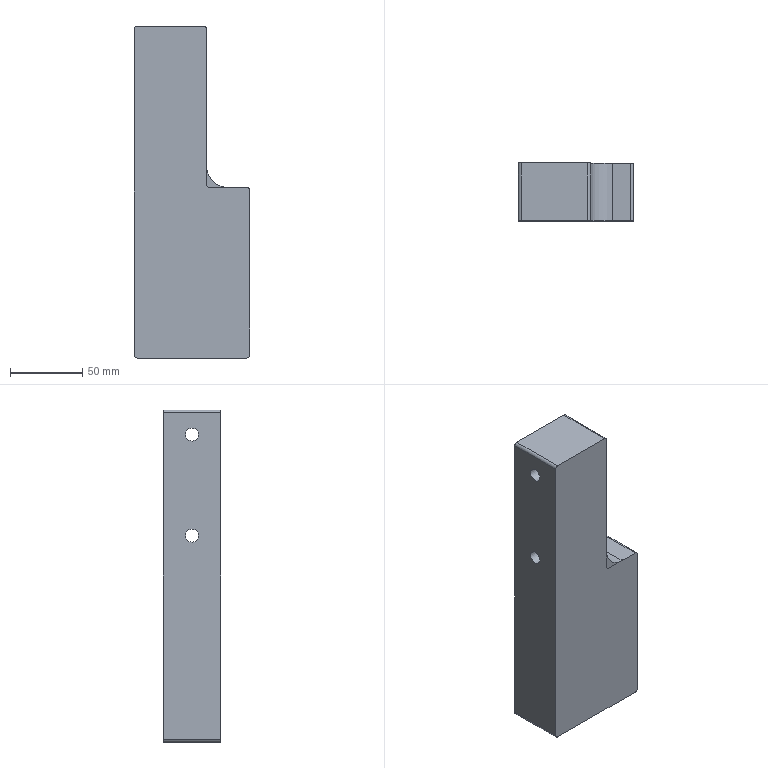NC program | NX | posted with a generic post | part box 80 x 40 x 230 mm
Lines 23 to 952 of 15398:
(PLANAR_MILL_COPY , TOOL : D16CU)
N44 T01 M6
N46 G53
N48 G17 G0 G90 X-126. Y-58. B0. C0. S1300 M3
N50 G43 Z50. H1
N52 Z-40.2
N54 G94 G1 Y-40. F2000.
N56 Y40.
N58 Y58.
N60 G0 Z50.
N62 X-125.8 Y-58.
N64 Z-40.2
N66 G1 Y-40.
N68 Y40.
N70 Y58.
N72 G0 Z50.
N74 X-125.6 Y-58.
N76 Z-40.2
N78 G1 Y-40.
N80 Y40.
N82 Y58.
N84 G0 Z50.
N86 X-125.4 Y-58.
N88 Z-40.2
N90 G1 Y-40.
N92 Y40.
N94 Y58.
N96 G0 Z50.
N98 X-125.2 Y-58.
N100 Z-40.2
N102 G1 Y-40.
N104 Y40.
N106 Y58.
N108 G0 Z50.
N110 X-125. Y-58.
N112 Z-40.2
N114 G1 Y-40.
N116 Y40.
N118 Y58.
N120 G0 Z50.
N122 X-124.8 Y-58.
N124 Z-40.2
N126 G1 Y-40.
N128 Y40.
N130 Y58.
N132 G0 Z50.
N134 X-124.6 Y-58.
N136 Z-40.2
N138 G1 Y-40.
N140 Y40.
N142 Y58.
N144 G0 Z50.
N146 X-124.4 Y-58.
N148 Z-40.2
N150 G1 Y-40.
N152 Y40.
N154 Y58.
N156 G0 Z50.
N158 X-124.2 Y-58.
N160 Z-40.2
N162 G1 Y-40.
N164 Y40.
N166 Y58.
N168 G0 Z50.
N170 X-124. Y-58.
N172 Z-40.2
N174 G1 Y-40.
N176 Y40.
N178 Y58.
N180 G0 Z50.
N182 X-123.8 Y-58.
N184 Z-40.2
N186 G1 Y-40.
N188 Y40.
N190 Y58.
N192 G0 Z50.
N194 X-123.6 Y-58.
N196 Z-40.2
N198 G1 Y-40.
N200 Y40.
N202 Y58.
N204 G0 Z50.
N206 X-123.4 Y-58.
N208 Z-40.2
N210 G1 Y-40.
N212 Y40.
N214 Y58.
N216 G0 Z50.
N218 X-123.2 Y-58.
N220 Z-40.2
N222 G1 Y-40.
N224 Y40.
N226 Y58.
N228 G0 Z50.
N230 X-123. Y-58.
N232 Z-40.2
N234 G1 Y-40.
N236 Y40.
N238 Y58.
N240 G0 Z50.
(PLANAR_MILL_COPY_COPY_2 , TOOL : D16CU)
N242 X126.
N244 Z-40.2
N246 G1 Y40.
N248 Y-40.
N250 Y-58.
N252 G0 Z50.
N254 X125.8 Y58.
N256 Z-40.2
N258 G1 Y40.
N260 Y-40.
N262 Y-58.
N264 G0 Z50.
N266 X125.6 Y58.
N268 Z-40.2
N270 G1 Y40.
N272 Y-40.
N274 Y-58.
N276 G0 Z50.
N278 X125.4 Y58.
N280 Z-40.2
N282 G1 Y40.
N284 Y-40.
N286 Y-58.
N288 G0 Z50.
N290 X125.2 Y58.
N292 Z-40.2
N294 G1 Y40.
N296 Y-40.
N298 Y-58.
N300 G0 Z50.
N302 X125. Y58.
N304 Z-40.2
N306 G1 Y40.
N308 Y-40.
N310 Y-58.
N312 G0 Z50.
N314 X124.8 Y58.
N316 Z-40.2
N318 G1 Y40.
N320 Y-40.
N322 Y-58.
N324 G0 Z50.
N326 X124.6 Y58.
N328 Z-40.2
N330 G1 Y40.
N332 Y-40.
N334 Y-58.
N336 G0 Z50.
N338 X124.4 Y58.
N340 Z-40.2
N342 G1 Y40.
N344 Y-40.
N346 Y-58.
N348 G0 Z50.
N350 X124.2 Y58.
N352 Z-40.2
N354 G1 Y40.
N356 Y-40.
N358 Y-58.
N360 G0 Z50.
N362 X124. Y58.
N364 Z-40.2
N366 G1 Y40.
N368 Y-40.
N370 Y-58.
N372 G0 Z50.
N374 X123.8 Y58.
N376 Z-40.2
N378 G1 Y40.
N380 Y-40.
N382 Y-58.
N384 G0 Z50.
N386 X123.6 Y58.
N388 Z-40.2
N390 G1 Y40.
N392 Y-40.
N394 Y-58.
N396 G0 Z50.
N398 X123.4 Y58.
N400 Z-40.2
N402 G1 Y40.
N404 Y-40.
N406 Y-58.
N408 G0 Z50.
N410 X123.2 Y58.
N412 Z-40.2
N414 G1 Y40.
N416 Y-40.
N418 Y-58.
N420 G0 Z50.
N422 X123. Y58.
N424 Z-40.2
N426 G1 Y40.
N428 Y-40.
N430 Y-58.
N432 G0 Z50.
(ADAPTIVE_MILLING , TOOL : D16CU)
N434 X-130.083 Y37.323
N436 Z-37.2
N438 G1 X-129.936 Y37.352 Z-38.137
N440 X-129.789 Y37.382 Z-38.508
N442 X-129.642 Y37.411 Z-38.78
N444 X-129.495 Y37.44 Z-39.
N446 X-129.348 Y37.47 Z-39.184
N448 X-129.2 Y37.499 Z-39.342
N450 X-129.053 Y37.528 Z-39.48
N452 X-128.906 Y37.558 Z-39.6
N454 X-128.759 Y37.587 Z-39.705
N456 X-128.612 Y37.617 Z-39.798
N458 X-128.465 Y37.646 Z-39.879
N460 X-128.318 Y37.675 Z-39.95
N462 X-128.171 Y37.705 Z-40.01
N464 X-128.024 Y37.734 Z-40.062
N466 X-127.877 Y37.763 Z-40.105
N468 X-127.73 Y37.793 Z-40.139
N470 X-127.582 Y37.822 Z-40.166
N472 X-127.435 Y37.852 Z-40.185
N474 X-127.288 Y37.881 Z-40.196
N476 X-127.141 Y37.91 Z-40.2
N478 X-124.066 Y38.536
N480 G3 X-122.931 Y40.211 R1.719
N482 X-122.789 Y44.171 R147.319
N484 G2 X-118.844 Y50.669 R8.892
N486 X-113.206 Y52.721 R13.027
N488 X-107.294 Y53.035 R46.448
N490 G1 X-100.978 Y53.05
N492 X113.642 Y53.039
N494 G2 X120.285 Y49.254 R8.846
N496 X122.447 Y43.589 R12.79
N498 X122.721 Y40.931 R89.136
N500 G1 X122.738 Y40.861
N502 X122.989 Y39.71
N504 G3 X123.222 Y39.159 R1.616
N506 G1 X124.137 Y37.782
N508 G3 X127.095 Y38.792 R1.616
N510 G1 X127.084 Y38.942 Z-40.196
N512 X127.073 Y39.091 Z-40.185
N514 X127.063 Y39.241 Z-40.166
N516 X127.052 Y39.391 Z-40.139
N518 X127.041 Y39.54 Z-40.105
N520 X127.031 Y39.69 Z-40.062
N522 X127.02 Y39.839 Z-40.01
N524 X127.009 Y39.989 Z-39.95
N526 X126.998 Y40.139 Z-39.879
N528 X126.988 Y40.288 Z-39.798
N530 X126.977 Y40.438 Z-39.705
N532 X126.966 Y40.587 Z-39.6
N534 X126.956 Y40.737 Z-39.48
N536 X126.945 Y40.887 Z-39.342
N538 X126.934 Y41.036 Z-39.184
N540 X126.924 Y41.186 Z-39.
N542 X126.913 Y41.336 Z-38.78
N544 X126.902 Y41.485 Z-38.508
N546 X126.891 Y41.635 Z-38.137
N548 X126.881 Y41.784 Z-37.2
N550 G0 Z50.
N552 X-127.141 Y34.005
N554 Z-37.2
N556 G1 Y34.155 Z-38.137
N558 Y34.305 Z-38.508
N560 Y34.455 Z-38.78
N562 Y34.605 Z-39.
N564 Y34.755 Z-39.184
N566 Y34.905 Z-39.342
N568 Y35.055 Z-39.48
N570 Y35.205 Z-39.6
N572 Y35.355 Z-39.705
N574 Y35.505 Z-39.798
N576 Y35.655 Z-39.879
N578 Y35.805 Z-39.95
N580 Y35.955 Z-40.01
N582 Y36.105 Z-40.062
N584 Y36.255 Z-40.105
N586 Y36.405 Z-40.139
N588 Y36.555 Z-40.166
N590 Y36.705 Z-40.185
N592 Y36.855 Z-40.196
N594 Y37.005 Z-40.2
N596 G2 X-125.042 Y38.536 R1.608
N598 G3 X-122.985 Y39.727 R1.608
N600 G1 X-122.905 Y40.093
N602 G3 X-122.649 Y42.805 R32.541
N604 G2 X-117.252 Y50.758 R10.401
N606 X-111.165 Y52.568 R15.926
N608 X-104.579 Y52.839 R65.062
N610 G1 X111.523 Y52.85
N612 G2 X120.343 Y47.721 R10.236
N614 X122.118 Y42.83 R15.137
N616 G1 X122.309 Y42.013
N618 X122.739 Y40.859
N620 G3 X122.969 Y40.443 R1.616
N622 G1 X124.075 Y38.993
N624 G3 X126.96 Y40.203 R1.616
N626 G1 X126.938 Y40.351 Z-40.196
N628 X126.917 Y40.5 Z-40.185
N630 X126.896 Y40.648 Z-40.166
N632 X126.874 Y40.797 Z-40.139
N634 X126.853 Y40.945 Z-40.105
N636 X126.832 Y41.094 Z-40.062
N638 X126.81 Y41.242 Z-40.01
N640 X126.789 Y41.391 Z-39.95
N642 X126.768 Y41.539 Z-39.879
N644 X126.746 Y41.687 Z-39.798
N646 X126.725 Y41.836 Z-39.705
N648 X126.703 Y41.984 Z-39.6
N650 X126.682 Y42.133 Z-39.48
N652 X126.661 Y42.281 Z-39.342
N654 X126.639 Y42.43 Z-39.184
N656 X126.618 Y42.578 Z-39.
N658 X126.597 Y42.727 Z-38.78
N660 X126.575 Y42.875 Z-38.508
N662 X126.554 Y43.024 Z-38.137
N664 X126.533 Y43.172 Z-37.2
N666 G0 Z50.
N668 X-127.141 Y33.531
N670 Z-37.2
N672 G1 Y33.681 Z-38.137
N674 Y33.831 Z-38.508
N676 Y33.981 Z-38.78
N678 Y34.131 Z-39.
N680 Y34.281 Z-39.184
N682 Y34.431 Z-39.342
N684 Y34.581 Z-39.48
N686 Y34.731 Z-39.6
N688 Y34.881 Z-39.705
N690 Y35.031 Z-39.798
N692 Y35.181 Z-39.879
N694 Y35.331 Z-39.95
N696 Y35.481 Z-40.01
N698 Y35.631 Z-40.062
N700 Y35.781 Z-40.105
N702 Y35.931 Z-40.139
N704 Y36.081 Z-40.166
N706 Y36.231 Z-40.185
N708 Y36.381 Z-40.196
N710 Y36.531 Z-40.2
N712 G2 X-126.131 Y38.029 R1.616
N714 G1 X-123.879 Y38.939
N716 G3 X-122.905 Y40.093 R1.616
N718 G1 X-122.762 Y40.753
N720 G2 X-122.047 Y44.075 R18.903
N722 X-115.562 Y50.959 R11.737
N724 X-109.335 Y52.422 R19.36
N726 X-101.388 Y52.646 R100.772
N728 G1 X109.893 Y52.65
N730 G2 X120.263 Y46.603 R11.274
N732 X121.662 Y43.27 R23.569
N734 G1 X121.707 Y43.179
N736 X122.233 Y42.215
N738 X122.312 Y42.005
N740 G3 X122.68 Y41.43 R1.616
N742 G1 X123.924 Y40.179
N744 G3 X126.649 Y41.661 R1.616
N746 G1 X126.617 Y41.808 Z-40.196
N748 X126.585 Y41.954 Z-40.185
N750 X126.553 Y42.101 Z-40.166
N752 X126.522 Y42.247 Z-40.139
N754 X126.49 Y42.394 Z-40.105
N756 X126.458 Y42.541 Z-40.062
N758 X126.426 Y42.687 Z-40.01
N760 X126.394 Y42.834 Z-39.95
N762 X126.362 Y42.98 Z-39.879
N764 X126.33 Y43.127 Z-39.798
N766 X126.298 Y43.273 Z-39.705
N768 X126.267 Y43.42 Z-39.6
N770 X126.235 Y43.567 Z-39.48
N772 X126.203 Y43.713 Z-39.342
N774 X126.171 Y43.86 Z-39.184
N776 X126.139 Y44.006 Z-39.
N778 X126.107 Y44.153 Z-38.78
N780 X126.075 Y44.299 Z-38.508
N782 X126.043 Y44.446 Z-38.137
N784 X126.012 Y44.593 Z-37.2
N786 G0 Z50.
N788 X-127.141 Y34.314
N790 Z-37.2
N792 G1 Y34.464 Z-38.137
N794 Y34.614 Z-38.508
N796 Y34.764 Z-38.78
N798 Y34.914 Z-39.
N800 Y35.064 Z-39.184
N802 Y35.214 Z-39.342
N804 Y35.364 Z-39.48
N806 Y35.514 Z-39.6
N808 Y35.664 Z-39.705
N810 Y35.814 Z-39.798
N812 Y35.964 Z-39.879
N814 Y36.114 Z-39.95
N816 Y36.264 Z-40.01
N818 Y36.414 Z-40.062
N820 Y36.564 Z-40.105
N822 Y36.714 Z-40.139
N824 Y36.864 Z-40.166
N826 Y37.014 Z-40.185
N828 Y37.164 Z-40.196
N830 Y37.314 Z-40.2
N832 G2 X-126.024 Y38.851 R1.616
N834 G1 X-123.842 Y39.56
N836 G3 X-122.706 Y40.981 R1.731
N838 G2 X-121.251 Y44.999 R18.01
N840 X-114.078 Y51.044 R13.024
N842 X-107.623 Y52.269 R23.31
N844 X-99.091 Y52.448 R141.201
N846 G1 X109.435 Y52.436
N848 G2 X119.743 Y46.454 R12.051
N850 X120.91 Y44.33 R96.581
N852 G1 X120.944 Y44.282
N854 X121.539 Y43.487
N856 X121.719 Y43.157
N858 G3 X122.072 Y42.717 R1.616
N860 G1 X123.544 Y41.425
N862 G3 X126.124 Y43.205 R1.616
N864 G1 X126.072 Y43.345 Z-40.196
N866 X126.019 Y43.486 Z-40.185
N868 X125.967 Y43.626 Z-40.166
N870 X125.914 Y43.767 Z-40.139
N872 X125.862 Y43.907 Z-40.105
N874 X125.809 Y44.048 Z-40.062
N876 X125.757 Y44.188 Z-40.01
N878 X125.705 Y44.329 Z-39.95
N880 X125.652 Y44.469 Z-39.879
N882 X125.6 Y44.61 Z-39.798
N884 X125.547 Y44.751 Z-39.705
N886 X125.495 Y44.891 Z-39.6
N888 X125.443 Y45.032 Z-39.48
N890 X125.39 Y45.172 Z-39.342
N892 X125.338 Y45.313 Z-39.184
N894 X125.285 Y45.453 Z-39.
N896 X125.233 Y45.594 Z-38.78
N898 X125.181 Y45.734 Z-38.508
N900 X125.128 Y45.875 Z-38.137
N902 X125.076 Y46.016 Z-37.2
N904 G0 Z50.
N906 X-127.34 Y35.371
N908 Z-37.2
N910 G1 X-127.329 Y35.521 Z-38.137
N912 X-127.318 Y35.67 Z-38.508
N914 X-127.307 Y35.82 Z-38.78
N916 X-127.297 Y35.969 Z-39.
N918 X-127.286 Y36.119 Z-39.184
N920 X-127.275 Y36.269 Z-39.342
N922 X-127.265 Y36.418 Z-39.48
N924 X-127.254 Y36.568 Z-39.6
N926 X-127.243 Y36.718 Z-39.705
N928 X-127.232 Y36.867 Z-39.798
N930 X-127.222 Y37.017 Z-39.879
N932 X-127.211 Y37.166 Z-39.95
N934 X-127.2 Y37.316 Z-40.01
N936 X-127.19 Y37.466 Z-40.062
N938 X-127.179 Y37.615 Z-40.105
N940 X-127.168 Y37.765 Z-40.139
N942 X-127.157 Y37.915 Z-40.166
N944 X-127.147 Y38.064 Z-40.185
N946 X-127.136 Y38.214 Z-40.196
N948 X-127.125 Y38.363 Z-40.2
N950 G2 X-125.439 Y39.862 R1.616
N952 G3 X-123.958 Y39.837 R9.425
N954 X-122.738 Y40.861 R1.616
N956 G1 X-122.232 Y42.217
N958 G2 X-117.625 Y48.579 R14.426
N960 X-110.684 Y51.571 R16.388
N962 X-103.768 Y52.191 R41.402
N964 X-88.811 Y52.25 R865.431
N966 G1 X108.227 Y52.239
N968 G2 X115.028 Y50.433 R13.46
N970 X119.522 Y46.004 R14.386
N972 G3 X120.083 Y45.235 R11.707
N974 G1 X120.672 Y44.646
N976 X120.956 Y44.266
N978 G3 X121.305 Y43.923 R1.616
N980 G1 X123.022 Y42.686
N982 G3 X125.385 Y44.771 R1.616
N984 G1 X125.313 Y44.903 Z-40.196
N986 X125.241 Y45.035 Z-40.185
N988 X125.169 Y45.166 Z-40.166
N990 X125.098 Y45.298 Z-40.139
N992 X125.026 Y45.43 Z-40.105
N994 X124.954 Y45.561 Z-40.062
N996 X124.882 Y45.693 Z-40.01
N998 X124.81 Y45.824 Z-39.95
N1000 X124.738 Y45.956 Z-39.879
N1002 X124.666 Y46.088 Z-39.798
N1004 X124.594 Y46.219 Z-39.705
N1006 X124.523 Y46.351 Z-39.6
N1008 X124.451 Y46.483 Z-39.48
N1010 X124.379 Y46.614 Z-39.342
N1012 X124.307 Y46.746 Z-39.184
N1014 X124.235 Y46.878 Z-39.
N1016 X124.163 Y47.009 Z-38.78
N1018 X124.091 Y47.141 Z-38.508
N1020 X124.019 Y47.273 Z-38.137
N1022 X123.948 Y47.404 Z-37.2
N1024 G0 Z50.
N1026 X-127.401 Y37.136
N1028 Z-37.2
N1030 G1 X-127.379 Y37.285 Z-38.137
N1032 X-127.358 Y37.433 Z-38.508
N1034 X-127.337 Y37.582 Z-38.78
N1036 X-127.315 Y37.73 Z-39.
N1038 X-127.294 Y37.879 Z-39.184
N1040 X-127.273 Y38.027 Z-39.342
N1042 X-127.251 Y38.175 Z-39.48
N1044 X-127.23 Y38.324 Z-39.6
N1046 X-127.208 Y38.472 Z-39.705
N1048 X-127.187 Y38.621 Z-39.798
N1050 X-127.166 Y38.769 Z-39.879
N1052 X-127.144 Y38.918 Z-39.95
N1054 X-127.123 Y39.066 Z-40.01
N1056 X-127.102 Y39.215 Z-40.062
N1058 X-127.08 Y39.363 Z-40.105
N1060 X-127.059 Y39.512 Z-40.139
N1062 X-127.038 Y39.66 Z-40.166
N1064 X-127.016 Y39.809 Z-40.185
N1066 X-126.995 Y39.957 Z-40.196
N1068 X-126.973 Y40.106 Z-40.2
N1070 G2 X-125.258 Y41.487 R1.616
N1072 G1 X-123.766 Y41.38
N1074 G3 X-122.232 Y42.217 R1.616
N1076 G1 X-121.538 Y43.488
N1078 G2 X-111.794 Y50.946 R15.769
N1080 X-104.869 Y51.918 R31.419
N1082 X-95.467 Y52.05 R208.938
N1084 G1 X107.184 Y52.039
N1086 G2 X113.556 Y50.686 R15.084
N1088 X118.495 Y46.75 R15.045
N1090 G3 X119.179 Y46.021 R7.07
N1092 G1 X119.648 Y45.67
N1094 X120.089 Y45.228
N1096 X120.44 Y44.962
N1098 X122.366 Y43.879
N1100 G3 X124.452 Y46.256 R1.616
N1102 G1 X124.362 Y46.376 Z-40.196
N1104 X124.272 Y46.496 Z-40.185
N1106 X124.182 Y46.616 Z-40.166
N1108 X124.092 Y46.736 Z-40.139
N1110 X124.002 Y46.856 Z-40.105
N1112 X123.913 Y46.976 Z-40.062
N1114 X123.823 Y47.096 Z-40.01
N1116 X123.733 Y47.217 Z-39.95
N1118 X123.643 Y47.337 Z-39.879
N1120 X123.553 Y47.457 Z-39.798
N1122 X123.463 Y47.577 Z-39.705
N1124 X123.373 Y47.697 Z-39.6
N1126 X123.283 Y47.817 Z-39.48
N1128 X123.194 Y47.937 Z-39.342
N1130 X123.104 Y48.057 Z-39.184
N1132 X123.014 Y48.177 Z-39.
N1134 X122.924 Y48.297 Z-38.78
N1136 X122.834 Y48.417 Z-38.508
N1138 X122.744 Y48.538 Z-38.137
N1140 X122.654 Y48.658 Z-37.2
N1142 G0 Z50.
N1144 X-127.438 Y38.986
N1146 Z-37.2
N1148 G1 X-127.396 Y39.13 Z-38.137
N1150 X-127.354 Y39.273 Z-38.508
N1152 X-127.312 Y39.417 Z-38.78
N1154 X-127.269 Y39.561 Z-39.
N1156 X-127.227 Y39.705 Z-39.184
N1158 X-127.185 Y39.849 Z-39.342
N1160 X-127.143 Y39.993 Z-39.48
N1162 X-127.1 Y40.137 Z-39.6
N1164 X-127.058 Y40.281 Z-39.705
N1166 X-127.016 Y40.425 Z-39.798
N1168 X-126.973 Y40.569 Z-39.879
N1170 X-126.931 Y40.713 Z-39.95
N1172 X-126.889 Y40.857 Z-40.01
N1174 X-126.847 Y41. Z-40.062
N1176 X-126.804 Y41.144 Z-40.105
N1178 X-126.762 Y41.288 Z-40.139
N1180 X-126.72 Y41.432 Z-40.166
N1182 X-126.677 Y41.576 Z-40.185
N1184 X-126.635 Y41.72 Z-40.196
N1186 X-126.593 Y41.864 Z-40.2
N1188 G2 X-124.9 Y43.018 R1.616
N1190 G1 X-122.975 Y42.847
N1192 G3 X-121.538 Y43.488 R1.616
N1194 G1 X-120.67 Y44.648
N1196 G2 X-113.539 Y49.974 R17.968
N1198 X-106.424 Y51.557 R24.811
N1200 X-97.782 Y51.841 R106.169
N1202 G1 X106.229 Y51.838
N1204 G2 X112.356 Y50.748 R16.847
N1206 X117.504 Y47.3 R16.134
N1208 G3 X118.262 Y46.662 R4.975
N1210 G1 X118.488 Y46.538
N1212 X119.189 Y46.014
N1214 X119.518 Y45.823
N1216 X121.646 Y44.907
N1218 G3 X123.428 Y47.534 R1.616
N1220 G1 X123.322 Y47.64 Z-40.196
N1222 X123.216 Y47.746 Z-40.185
N1224 X123.11 Y47.852 Z-40.166
N1226 X123.004 Y47.958 Z-40.139
N1228 X122.898 Y48.064 Z-40.105
N1230 X122.792 Y48.17 Z-40.062
N1232 X122.686 Y48.276 Z-40.01
N1234 X122.58 Y48.382 Z-39.95
N1236 X122.474 Y48.488 Z-39.879
N1238 X122.368 Y48.595 Z-39.798
N1240 X122.262 Y48.701 Z-39.705
N1242 X122.155 Y48.807 Z-39.6
N1244 X122.049 Y48.913 Z-39.48
N1246 X121.943 Y49.019 Z-39.342
N1248 X121.837 Y49.125 Z-39.184
N1250 X121.731 Y49.231 Z-39.
N1252 X121.625 Y49.337 Z-38.78
N1254 X121.519 Y49.443 Z-38.508
N1256 X121.413 Y49.549 Z-38.137
N1258 X121.307 Y49.655 Z-37.2
N1260 G0 Z50.
N1262 X-127.21 Y40.902
N1264 Z-37.2
N1266 G1 X-127.147 Y41.039 Z-38.137
N1268 X-127.085 Y41.175 Z-38.508
N1270 X-127.023 Y41.312 Z-38.78
N1272 X-126.96 Y41.448 Z-39.
N1274 X-126.898 Y41.584 Z-39.184
N1276 X-126.836 Y41.721 Z-39.342
N1278 X-126.773 Y41.857 Z-39.48
N1280 X-126.711 Y41.994 Z-39.6
N1282 X-126.649 Y42.13 Z-39.705
N1284 X-126.586 Y42.267 Z-39.798
N1286 X-126.524 Y42.403 Z-39.879
N1288 X-126.462 Y42.539 Z-39.95
N1290 X-126.4 Y42.676 Z-40.01
N1292 X-126.337 Y42.812 Z-40.062
N1294 X-126.275 Y42.949 Z-40.105
N1296 X-126.213 Y43.085 Z-40.139
N1298 X-126.15 Y43.222 Z-40.166
N1300 X-126.088 Y43.358 Z-40.185
N1302 X-126.026 Y43.495 Z-40.196
N1304 X-125.963 Y43.631 Z-40.2
N1306 G2 X-124.228 Y44.554 R1.616
N1308 G1 X-122.078 Y44.196
N1310 G3 X-120.67 Y44.648 R1.616
N1312 G1 X-119.646 Y45.672
N1314 G2 X-113.341 Y49.691 R21.533
N1316 X-105.927 Y51.34 R26.248
N1318 X-96.76 Y51.641 R110.456
N1320 G1 X105.386 Y51.637
N1322 G2 X111.667 Y50.593 R18.387
N1324 X116.701 Y47.596 R18.342
N1326 G1 X117.216 Y47.233
N1328 X118.271 Y46.657
N1330 G3 X121.012 Y45.767 R30.293
N1332 X122.373 Y48.576 R1.616
N1334 G1 X122.26 Y48.674 Z-40.196
N1336 X122.147 Y48.772 Z-40.185
N1338 X122.033 Y48.871 Z-40.166
N1340 X121.92 Y48.969 Z-40.139
N1342 X121.806 Y49.067 Z-40.105
N1344 X121.693 Y49.165 Z-40.062
N1346 X121.58 Y49.264 Z-40.01
N1348 X121.466 Y49.362 Z-39.95
N1350 X121.353 Y49.46 Z-39.879
N1352 X121.24 Y49.558 Z-39.798
N1354 X121.126 Y49.657 Z-39.705
N1356 X121.013 Y49.755 Z-39.6
N1358 X120.9 Y49.853 Z-39.48
N1360 X120.786 Y49.951 Z-39.342
N1362 X120.673 Y50.05 Z-39.184
N1364 X120.56 Y50.148 Z-39.
N1366 X120.446 Y50.246 Z-38.78
N1368 X120.333 Y50.344 Z-38.508
N1370 X120.22 Y50.442 Z-38.137
N1372 X120.106 Y50.541 Z-37.2
N1374 G0 Z50.
N1376 X-121.181 Y49.781
N1378 Z-37.2
N1380 G1 X-121.287 Y49.675 Z-38.137
N1382 X-121.393 Y49.569 Z-38.508
N1384 X-121.499 Y49.463 Z-38.78
N1386 X-121.605 Y49.357 Z-39.
N1388 X-121.711 Y49.251 Z-39.184
N1390 X-121.817 Y49.144 Z-39.342
N1392 X-121.923 Y49.038 Z-39.48
N1394 X-122.029 Y48.932 Z-39.6
N1396 X-122.135 Y48.826 Z-39.705
N1398 X-122.242 Y48.72 Z-39.798
N1400 X-122.348 Y48.614 Z-39.879
N1402 X-122.454 Y48.508 Z-39.95
N1404 X-122.56 Y48.402 Z-40.01
N1406 X-122.666 Y48.296 Z-40.062
N1408 X-122.772 Y48.19 Z-40.105
N1410 X-122.878 Y48.084 Z-40.139
N1412 X-122.984 Y47.978 Z-40.166
N1414 X-123.09 Y47.872 Z-40.185
N1416 X-123.196 Y47.766 Z-40.196
N1418 X-123.302 Y47.66 Z-40.2
N1420 G3 X-121.709 Y44.965 R1.616
N1422 G1 X-119.981 Y45.478
N1424 X-119.646 Y45.672
N1426 X-118.487 Y46.539
N1428 G2 X-112.189 Y49.787 R25.918
N1430 X-104.221 Y51.225 R31.349
N1432 X-93.962 Y51.448 R167.743
N1434 G1 X104.418 Y51.439
N1436 G2 X110.668 Y50.553 R20.751
N1438 X115.69 Y47.987 R19.877
N1440 G3 X116.551 Y47.481 R4.058
N1442 G1 X117.217 Y47.232
N1444 G3 X120.032 Y46.63 R74.076
N1446 X121.147 Y49.533 R1.616
N1448 G1 X121.027 Y49.623 Z-40.196
N1450 X120.907 Y49.713 Z-40.185
N1452 X120.787 Y49.803 Z-40.166
N1454 X120.667 Y49.893 Z-40.139
N1456 X120.547 Y49.983 Z-40.105
N1458 X120.427 Y50.073 Z-40.062
N1460 X120.307 Y50.162 Z-40.01
N1462 X120.187 Y50.252 Z-39.95
N1464 X120.067 Y50.342 Z-39.879
N1466 X119.947 Y50.432 Z-39.798
N1468 X119.827 Y50.522 Z-39.705
N1470 X119.706 Y50.612 Z-39.6
N1472 X119.586 Y50.702 Z-39.48
N1474 X119.466 Y50.792 Z-39.342
N1476 X119.346 Y50.882 Z-39.184
N1478 X119.226 Y50.972 Z-39.
N1480 X119.106 Y51.062 Z-38.78
N1482 X118.986 Y51.151 Z-38.508
N1484 X118.866 Y51.241 Z-38.137
N1486 X118.746 Y51.331 Z-37.2
N1488 G0 Z50.
N1490 X-120.492 Y50.469
N1492 Z-37.2
N1494 G1 X-120.599 Y50.363 Z-38.137
N1496 X-120.705 Y50.257 Z-38.508
N1498 X-120.811 Y50.151 Z-38.78
N1500 X-120.917 Y50.045 Z-39.
N1502 X-121.023 Y49.939 Z-39.184
N1504 X-121.129 Y49.833 Z-39.342
N1506 X-121.235 Y49.727 Z-39.48
N1508 X-121.341 Y49.621 Z-39.6
N1510 X-121.447 Y49.515 Z-39.705
N1512 X-121.553 Y49.408 Z-39.798
N1514 X-121.659 Y49.302 Z-39.879
N1516 X-121.765 Y49.196 Z-39.95
N1518 X-121.871 Y49.09 Z-40.01
N1520 X-121.978 Y48.984 Z-40.062
N1522 X-122.084 Y48.878 Z-40.105
N1524 X-122.19 Y48.772 Z-40.139
N1526 X-122.296 Y48.666 Z-40.166
N1528 X-122.402 Y48.56 Z-40.185
N1530 X-122.508 Y48.454 Z-40.196
N1532 X-122.614 Y48.348 Z-40.2
N1534 G3 X-120.951 Y45.675 R1.616
N1536 X-118.487 Y46.539 R42.668
N1538 G1 X-117.215 Y47.233
N1540 G2 X-109.032 Y50.335 R28.812
N1542 X-101.048 Y51.149 R47.484
N1544 X-89.506 Y51.251 R358.335
N1546 G1 X103.79 Y51.235
N1548 G2 X110.288 Y50.312 R22.041
N1550 X115.127 Y48.039 R24.521
N1552 G3 X115.771 Y47.758 R2.109
N1554 G1 X115.861 Y47.738
N1556 X116.563 Y47.476
N1558 G3 X117.211 Y47.376 R1.616
N1560 G1 X118.88 Y47.462
N1562 G3 X119.572 Y50.494 R1.616
N1564 G1 X119.44 Y50.566 Z-40.196
N1566 X119.309 Y50.638 Z-40.185
N1568 X119.177 Y50.71 Z-40.166
N1570 X119.045 Y50.781 Z-40.139
N1572 X118.914 Y50.853 Z-40.105
N1574 X118.782 Y50.925 Z-40.062
N1576 X118.651 Y50.997 Z-40.01
N1578 X118.519 Y51.069 Z-39.95
N1580 X118.387 Y51.141 Z-39.879
N1582 X118.256 Y51.213 Z-39.798
N1584 X118.124 Y51.285 Z-39.705
N1586 X117.992 Y51.357 Z-39.6
N1588 X117.861 Y51.429 Z-39.48
N1590 X117.729 Y51.5 Z-39.342
N1592 X117.597 Y51.572 Z-39.184
N1594 X117.466 Y51.644 Z-39.
N1596 X117.334 Y51.716 Z-38.78
N1598 X117.202 Y51.788 Z-38.508
N1600 X117.071 Y51.86 Z-38.137
N1602 X116.939 Y51.932 Z-37.2
N1604 G0 Z50.
N1606 X-118.736 Y51.337
N1608 Z-37.2
N1610 G1 X-118.857 Y51.248 Z-38.137
N1612 X-118.977 Y51.158 Z-38.508
N1614 X-119.097 Y51.068 Z-38.78
N1616 X-119.217 Y50.978 Z-39.
N1618 X-119.337 Y50.888 Z-39.184
N1620 X-119.457 Y50.798 Z-39.342
N1622 X-119.577 Y50.708 Z-39.48
N1624 X-119.697 Y50.618 Z-39.6
N1626 X-119.817 Y50.529 Z-39.705
N1628 X-119.937 Y50.439 Z-39.798
N1630 X-120.057 Y50.349 Z-39.879
N1632 X-120.178 Y50.259 Z-39.95
N1634 X-120.298 Y50.169 Z-40.01
N1636 X-120.418 Y50.079 Z-40.062
N1638 X-120.538 Y49.989 Z-40.105
N1640 X-120.658 Y49.899 Z-40.139
N1642 X-120.778 Y49.809 Z-40.166
N1644 X-120.898 Y49.72 Z-40.185
N1646 X-121.018 Y49.63 Z-40.196
N1648 X-121.138 Y49.54 Z-40.2
N1650 G3 X-119.838 Y46.664 R1.616
N1652 X-117.215 Y47.233 R100.24
N1654 G1 X-116.841 Y47.373
N1656 G2 X-111.853 Y49.323 R56.419
N1658 X-102.905 Y50.834 R37.075
N1660 X-92.453 Y51.047 R178.715
N1662 G1 X102.834 Y51.038
N1664 G2 X109.334 Y50.254 R25.044
N1666 X114.299 Y48.218 R27.133
N1668 G3 X115.061 Y47.913 R3.097
N1670 G1 X115.794 Y47.753
N1672 G3 X116.27 Y47.722 R1.616
N1674 G1 X118.113 Y47.873
N1676 G3 X118.652 Y50.954 R1.616
N1678 G1 X118.515 Y51.016 Z-40.196
N1680 X118.379 Y51.078 Z-40.185
N1682 X118.242 Y51.141 Z-40.166
N1684 X118.106 Y51.203 Z-40.139
N1686 X117.969 Y51.265 Z-40.105
N1688 X117.833 Y51.328 Z-40.062
N1690 X117.697 Y51.39 Z-40.01
N1692 X117.56 Y51.452 Z-39.95
N1694 X117.424 Y51.515 Z-39.879
N1696 X117.287 Y51.577 Z-39.798
N1698 X117.151 Y51.639 Z-39.705
N1700 X117.014 Y51.702 Z-39.6
N1702 X116.878 Y51.764 Z-39.48
N1704 X116.741 Y51.826 Z-39.342
N1706 X116.605 Y51.889 Z-39.184
N1708 X116.469 Y51.951 Z-39.
N1710 X116.332 Y52.013 Z-38.78
N1712 X116.196 Y52.076 Z-38.508
N1714 X116.059 Y52.138 Z-38.137
N1716 X115.923 Y52.2 Z-37.2
N1718 G0 Z50.
N1720 X-117.28 Y51.745
N1722 Z-37.2
N1724 G1 X-117.411 Y51.673 Z-38.137
N1726 X-117.543 Y51.601 Z-38.508
N1728 X-117.675 Y51.53 Z-38.78
N1730 X-117.806 Y51.458 Z-39.
N1732 X-117.938 Y51.386 Z-39.184
N1734 X-118.07 Y51.314 Z-39.342
N1736 X-118.201 Y51.242 Z-39.48
N1738 X-118.333 Y51.17 Z-39.6
N1740 X-118.465 Y51.098 Z-39.705
N1742 X-118.596 Y51.026 Z-39.798
N1744 X-118.728 Y50.955 Z-39.879
N1746 X-118.86 Y50.883 Z-39.95
N1748 X-118.991 Y50.811 Z-40.01
N1750 X-119.123 Y50.739 Z-40.062
N1752 X-119.255 Y50.667 Z-40.105
N1754 X-119.386 Y50.595 Z-40.139
N1756 X-119.518 Y50.523 Z-40.166
N1758 X-119.65 Y50.451 Z-40.185
N1760 X-119.781 Y50.38 Z-40.196
N1762 X-119.913 Y50.308 Z-40.2
N1764 G3 X-119.141 Y47.273 R1.616
N1766 G1 X-117.215 Y47.282
N1768 X-116.841 Y47.373
N1770 X-115.859 Y47.739
N1772 G2 X-111.005 Y49.32 R92.437
N1774 X-101.529 Y50.68 R43.503
N1776 X-90.184 Y50.85 R240.151
N1778 G1 X102.095 Y50.837
N1780 G2 X108.872 Y50.056 R27.233
N1782 X113.654 Y48.276 R33.114
N1784 G3 X114.416 Y48.049 R2.222
N1786 G1 X114.446 Y48.046
N1788 X115.081 Y47.908
N1790 G3 X115.673 Y47.89 R1.616
N1792 G1 X117.468 Y48.17
N1794 G3 X117.785 Y51.281 R1.616
N1796 G1 X117.644 Y51.333 Z-40.196
N1798 X117.504 Y51.385 Z-40.185
N1800 X117.363 Y51.438 Z-40.166
N1802 X117.223 Y51.49 Z-40.139
N1804 X117.082 Y51.543 Z-40.105
N1806 X116.941 Y51.595 Z-40.062
N1808 X116.801 Y51.648 Z-40.01
N1810 X116.66 Y51.7 Z-39.95
N1812 X116.52 Y51.752 Z-39.879
N1814 X116.379 Y51.805 Z-39.798
N1816 X116.239 Y51.857 Z-39.705
N1818 X116.098 Y51.91 Z-39.6
N1820 X115.958 Y51.962 Z-39.48
N1822 X115.817 Y52.015 Z-39.342
N1824 X115.677 Y52.067 Z-39.184
N1826 X115.536 Y52.119 Z-39.
N1828 X115.396 Y52.172 Z-38.78
N1830 X115.255 Y52.224 Z-38.508
N1832 X115.114 Y52.277 Z-38.137
N1834 X114.974 Y52.329 Z-37.2
N1836 G0 Z50.
N1838 X-116.001 Y52.164
N1840 Z-37.2
N1842 G1 X-116.137 Y52.102 Z-38.137
N1844 X-116.273 Y52.04 Z-38.508
N1846 X-116.41 Y51.977 Z-38.78
N1848 X-116.546 Y51.915 Z-39.
N1850 X-116.683 Y51.853 Z-39.184
N1852 X-116.819 Y51.79 Z-39.342
N1854 X-116.956 Y51.728 Z-39.48
N1856 X-117.092 Y51.666 Z-39.6
N1858 X-117.229 Y51.603 Z-39.705
N1860 X-117.365 Y51.541 Z-39.798
N1862 X-117.501 Y51.479 Z-39.879
N1864 X-117.638 Y51.417 Z-39.95
N1866 X-117.774 Y51.354 Z-40.01
N1868 X-117.911 Y51.292 Z-40.062
N1870 X-118.047 Y51.23 Z-40.105
N1872 X-118.184 Y51.167 Z-40.139
N1874 X-118.32 Y51.105 Z-40.166
N1876 X-118.457 Y51.043 Z-40.185
N1878 X-118.593 Y50.98 Z-40.196
N1880 X-118.73 Y50.918 Z-40.2
N1882 G3 X-118.171 Y47.836 R1.616
N1884 X-116.009 Y47.714 R25.075